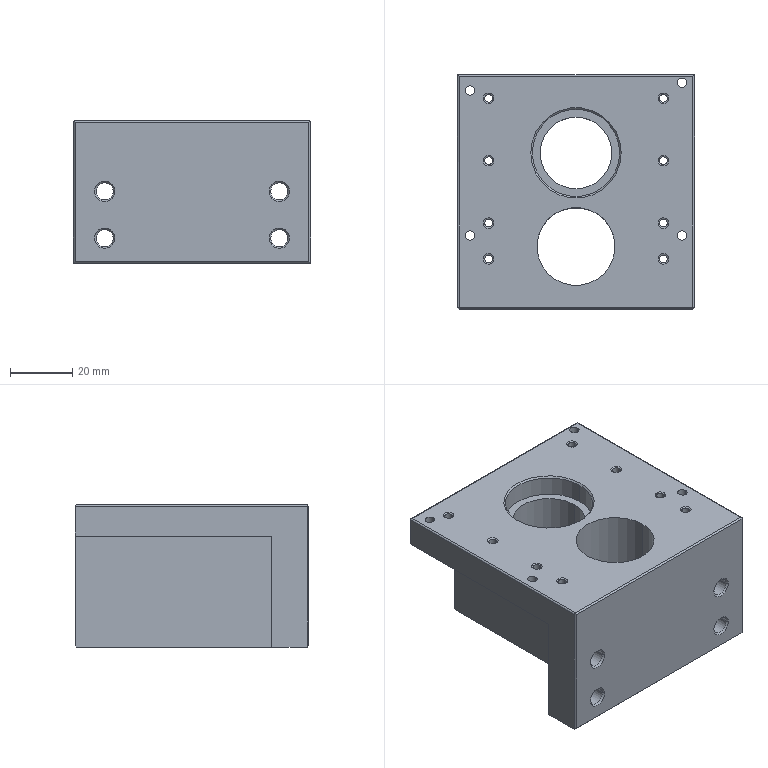Part | NX | 1 solid | 102 faces | box 76 x 75 x 45.6 mm | volume 124165 mm3 | cylinder 47 | cone 36 | plane 19 | commonest cylinder face diameters 2.5 x20 3 x8 5.5 x8 28 x4 1 x3 23 x2